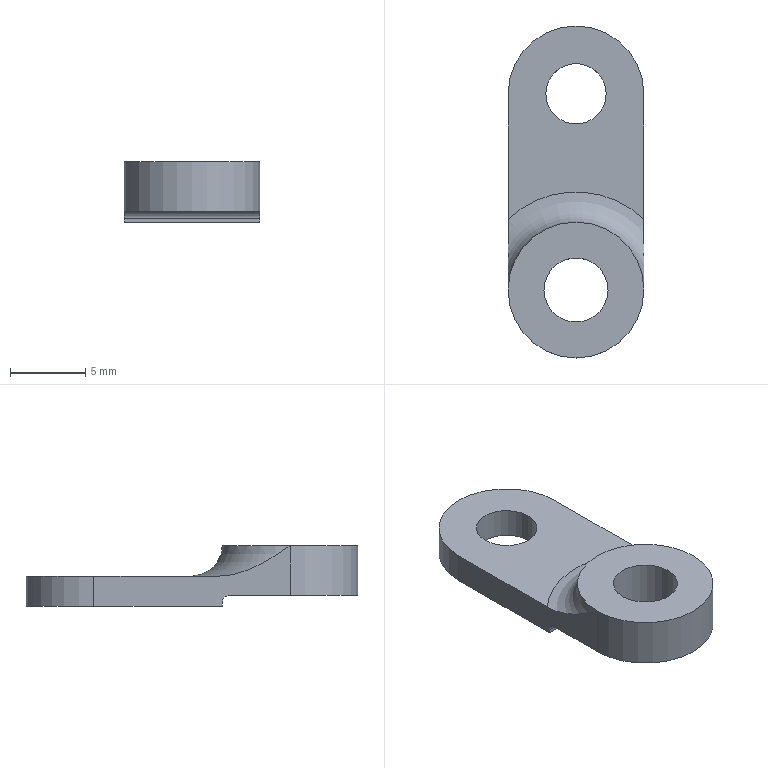NC program | NX | posted with a generic post | part box 9 x 22 x 4 mm
Whole program:
N10 G17 G21 G94 G90
(ADAPTIVE_MILLING_1 , TOOL : D10-30-D10-75-3T-FINISH)
N12 T01 M6
N14 G54
N16 G17 G0 G90 X3.609 Y-21.526 S4500 M3
N18 G43 Z1.15 H1
N20 G94 G1 X3.616 Y-21.377 Z0.213 F1500.
N22 X3.623 Y-21.227 Z-0.158
N24 X3.63 Y-21.077 Z-0.43
N26 X3.637 Y-20.927 Z-0.65
N28 X3.645 Y-20.777 Z-0.834
N30 X3.652 Y-20.627 Z-0.992
N32 X3.659 Y-20.478 Z-1.13
N34 X3.666 Y-20.328 Z-1.25
N36 X3.674 Y-20.178 Z-1.355
N38 X3.681 Y-20.028 Z-1.448
N40 X3.688 Y-19.878 Z-1.529
N42 X3.695 Y-19.728 Z-1.6
N44 X3.702 Y-19.579 Z-1.66
N46 X3.71 Y-19.429 Z-1.712
N48 X3.717 Y-19.279 Z-1.755
N50 X3.724 Y-19.129 Z-1.789
N52 X3.731 Y-18.979 Z-1.816
N54 X3.738 Y-18.83 Z-1.835
N56 X3.746 Y-18.68 Z-1.846
N58 X3.753 Y-18.53 Z-1.85
N60 X3.825 Y-17.028
N62 G3 X3.076 Y-16.003 R1.01
N64 X0.037 Y-15.742 R15.676
N66 X-13.568 Y-15.694 R849.737
N68 G2 X-17.871 Y-13.148 R5.709
N70 X-19.406 Y-8.918 R9.675
N72 X-19.687 Y-3.38 R43.207
N74 G1 X-19.688 Y9.665
N76 G2 X-17.106 Y13.908 R5.731
N78 X-12.87 Y15.415 R9.753
N80 X-7.406 Y15.687 R43.942
N82 G1 X-1.406 Y15.7
N84 X13.483 Y15.697
N86 G2 X17.786 Y13.257 R5.676
N88 X19.396 Y8.976 R9.508
N90 X19.687 Y3.363 R42.446
N92 G1 X19.688 Y-9.657
N94 G2 X17.068 Y-13.92 R5.764
N96 X12.704 Y-15.435 R9.931
N98 X6.975 Y-15.69 R48.838
N100 X1.55 Y-15.516 R62.965
N102 G3 X-7.344 Y-15.401 R225.311
N104 G2 X-12.292 Y-15.371 R114.167
N106 X-17.685 Y-11.8 R6.997
N108 X-19.122 Y-7.137 R12.027
N110 X-19.389 Y-0.921 R56.646
N112 G1 X-19.384 Y8.116
N114 G2 X-15.838 Y13.667 R6.965
N116 X-11.143 Y15.123 R11.979
N118 X-4.964 Y15.389 R56.383
N120 G1 X0.398 Y15.399
N122 G2 X12.166 Y15.38 R746.145
N124 X17.651 Y11.854 R6.984
N126 X19.118 Y7.163 R11.937
N128 X19.39 Y0.872 R56.383
N130 X19.38 Y-8.166 R448.832
N132 X15.843 Y-13.657 R6.985
N134 X11.184 Y-15.115 R11.931
N136 X2.542 Y-15.26 R51.547
N138 G3 X-10.343 Y-15.099 R304.983
N140 G2 X-17.445 Y-10.754 R7.845
N142 X-18.825 Y-5.837 R13.76
N144 X-19.089 Y0.755 R65.04
N146 X-19.07 Y7.017 R168.466
N148 X-14.85 Y13.396 R7.799
N150 X-9.944 Y14.813 R13.522
N152 X-3.766 Y15.086 R59.319
N154 G1 X1.184 Y15.099
N156 G2 X10.892 Y15.077 R558.443
N158 X17.433 Y10.77 R7.825
N160 X18.835 Y5.741 R13.864
N162 X19.089 Y-0.776 R66.532
N164 X19.07 Y-7.001 R166.156
N166 X14.828 Y-13.403 R7.812
N168 X9.805 Y-14.828 R13.709
N170 X3.25 Y-14.975 R44.243
N172 G3 X-9.446 Y-14.791 R366.794
N174 G2 X-17.181 Y-9.859 R8.509
N176 X-18.526 Y-4.733 R15.228
N178 X-18.791 Y2.459 R74.868
N180 X-18.73 Y6.357 R43.18
N182 X-13.925 Y13.15 R8.444
N184 X-8.659 Y14.535 R15.239
N186 X-1.166 Y14.792 R79.941
N188 X9.766 Y14.776 R610.284
N190 X17.168 Y9.88 R8.478
N192 X18.527 Y4.721 R15.214
N194 X18.791 Y-2.546 R75.709
N196 X18.735 Y-6.294 R44.285
N198 X13.934 Y-13.141 R8.447
N200 X8.629 Y-14.533 R15.121
N202 X2.297 Y-14.634 R51.252
N204 G3 X-8.591 Y-14.486 R621.68
N206 G2 X-14.357 Y-12.437 R9.223
N208 X-17.556 Y-7.328 R10.375
N210 X-18.376 Y-1.776 R23.819
N212 X-18.446 Y5.159 R79.772
N214 X-13.175 Y12.851 R8.97
N216 X-7.747 Y14.228 R16.352
N218 X-0.255 Y14.491 R81.917
N220 X8.904 Y14.467 R318.621
N222 X16.881 Y9.104 R9.014
N224 X18.239 Y3.634 R16.616
N226 X18.441 Y-5.208 R73.933
N228 X13.26 Y-12.806 R8.955
N230 X7.579 Y-14.222 R15.864
N232 X1.357 Y-14.304 R62.276
N234 G1 X-7.7 Y-14.185
N236 G2 X-13.037 Y-12.649 R10.181
N238 X-16.989 Y-7.401 R10.172
N240 X-18.016 Y-1.811 R21.157
N242 X-18.124 Y4.409 R54.641
N244 X-12.505 Y12.539 R9.397
N246 X-6.961 Y13.917 R17.224
N248 X0.493 Y14.188 R82.102
N250 X7.955 Y14.167 R255.277
N252 X13.789 Y12.098 R9.741
N254 X17.187 Y6.797 R10.701
N256 X18.058 Y1.139 R24.061
N258 X18.114 Y-4.52 R50.155
N260 X12.518 Y-12.529 R9.389
N262 X6.854 Y-13.884 R16.496
N264 X0.632 Y-13.984 R67.965
N266 X-7.298 Y-13.866 R417.053
N268 X-12.956 Y-11.994 R10.359
N270 X-16.735 Y-6.581 R10.758
N272 X-17.724 Y-0.831 R22.945
N274 X-17.747 Y4.225 R31.546
N276 X-12.089 Y12.127 R9.683
N278 X-6.599 Y13.567 R17.197
N280 X0.853 Y13.884 R73.619
N282 X7.452 Y13.845 R128.638
N284 X13.465 Y11.589 R10.083
N286 X16.863 Y6.169 R11.132
N288 X17.76 Y0.212 R25.388
N290 X17.721 Y-4.432 R27.272
N292 X11.998 Y-12.163 R9.675
N294 X6.19 Y-13.546 R16.957
N296 X-0.144 Y-13.666 R72.401
N298 X-6.705 Y-13.556 R181.339
N300 X-12.401 Y-11.689 R10.836
N302 X-16.338 Y-6.213 R10.97
N304 X-17.413 Y-0.176 R23.083
N306 X-17.262 Y4.571 R19.011
N308 X-11.718 Y11.708 R9.908
N310 X-6.024 Y13.245 R17.408
N312 X1.352 Y13.58 R71.272
N314 X7.05 Y13.514 R75.615
N316 X13.379 Y10.889 R10.304
N318 X16.613 Y5.329 R11.781
N320 X17.415 Y-3.484 R27.912
N322 X11.398 Y-11.847 R9.957
N324 X5.585 Y-13.209 R17.564
N326 X-0.936 Y-13.352 R75.645
N328 X-6.329 Y-13.232 R83.502
N330 X-12.306 Y-11.063 R10.975
N332 X-16.079 Y-5.474 R11.471
N334 X-17.032 Y3.159 R22.882
N336 X-11.108 Y11.417 R10.166
N338 X-5.332 Y12.941 R18.118
N340 X2.119 Y13.279 R73.326
N342 X6.989 Y13.144 R40.014
N344 X15.529 Y6.877 R10.403
N346 X16.972 Y1.037 R18.895
N348 X16.892 Y-4.082 R17.762
N350 X11.009 Y-11.443 R10.102
N352 X5.13 Y-12.865 R17.729
N354 X-2.627 Y-13.035 R85.322
N356 X-7.334 Y-12.708 R25.883
N358 X-15.176 Y-6.439 R10.653
N360 X-16.617 Y2.954 R18.961
N362 X-10.779 Y10.999 R10.29
N364 X-4.831 Y12.618 R18.184
N366 X5.693 Y12.9 R71.264
N368 X11.675 Y10.838 R11.344
N370 X15.637 Y5.284 R11.505
N372 X16.633 Y-2.807 R19.358
N374 X10.702 Y-11.008 R10.22
N376 X4.842 Y-12.508 R17.579
N378 X-5.235 Y-12.613 R70.379
N380 X-11.249 Y-10.496 R11.72
N382 X-15.352 Y-4.682 R11.811
N384 X-16.208 Y2.559 R16.692
N386 X-10.572 Y10.522 R10.343
N388 X-4.661 Y12.255 R17.668
N390 X5.184 Y12.579 R57.922
N392 X11.27 Y10.465 R11.606
N394 X15.351 Y4.67 R11.789
N396 X16.194 Y-2.645 R16.581
N398 X10.306 Y-10.62 R10.288
N400 X4.42 Y-12.166 R17.689
N402 X-4.681 Y-12.303 R57.154
N404 X-10.743 Y-10.209 R12.052
N406 X-14.998 Y-4.28 R11.945
N408 X-15.715 Y2.627 R14.386
N410 X-10.273 Y10.094 R10.362
N412 X-4.272 Y11.922 R17.545
N414 X4.821 Y12.243 R47.152
N416 X11.159 Y9.877 R11.662
N418 X14.712 Y5.046 R11.986
N420 X15.473 Y3.549 R13.977
N422 G1 X15.914 Y2.119
N424 X16.129 Y0.637
N426 G2 X14.991 Y-5.192 R13.078
N428 X9.203 Y-10.564 R10.913
N430 X3.076 Y-11.919 R20.103
N432 X-4.527 Y-11.951 R44.217
N434 X-10.975 Y-9.366 R11.848
N436 X-14.948 Y-2.866 R12.535
N438 X-14.877 Y3.864 R11.824
N440 X-9.536 Y9.902 R10.556
N442 X-3.587 Y11.631 R18.295
N444 X4.494 Y11.898 R38.875
N446 X11.015 Y9.308 R11.683
N448 X13.046 Y7.074 R11.835
N450 G1 X13.959 Y6.122
N452 X14.816 Y4.895
N454 X15.473 Y3.549
N456 X15.914 Y2.119
N458 X16.129 Y0.637
N460 X16.112 Y-0.86
N462 X15.863 Y-2.336
N464 X15.389 Y-3.757
N466 G2 X12.911 Y-7.448 R13.968
N468 X6.674 Y-10.926 R13.162
N470 X0.1 Y-11.738 R29.977
N472 X-5.428 Y-11.416 R24.678
N474 X-14. Y-4.23 R11.461
N476 X-14.533 Y3.119 R11.506
N478 X-9.349 Y9.421 R10.423
N480 X-3.363 Y11.277 R17.751
N482 X4.228 Y11.541 R32.406
N484 X11.338 Y8.327 R11.784
N486 G1 X11.731 Y8.109
N488 G2 X13.052 Y7.067 R12.874
N490 G1 X13.959 Y6.122
N492 X14.816 Y4.895
N494 X15.473 Y3.549
N496 X15.914 Y2.119
N498 X16.129 Y0.637
N500 X16.112 Y-0.86
N502 X15.863 Y-2.336
N504 X15.389 Y-3.757
N506 X14.701 Y-5.086
N508 X13.815 Y-6.293
N510 G2 X12.548 Y-7.512 R16.368
N512 X4.238 Y-11.016 R17.399
N514 X-3.911 Y-11.26 R31.391
N516 X-11.036 Y-7.884 R11.805
N518 X-14.332 Y1.255 R11.547
N520 X-9.499 Y8.725 R10.08
N522 X-3.562 Y10.851 R16.39
N524 X3.945 Y11.179 R27.757
N526 X9.599 Y9.119 R12.485
N528 X11.375 Y8.304 R8.087
N530 G1 X11.731 Y8.109
N532 X12.923 Y7.202
N534 X13.959 Y6.122
N536 X14.816 Y4.895
N538 X15.473 Y3.549
N540 X15.914 Y2.119
N542 X16.129 Y0.637
N544 X16.112 Y-0.86
N546 X15.863 Y-2.336
N548 X15.389 Y-3.757
N550 X14.701 Y-5.086
N552 X13.815 Y-6.293
N554 X12.754 Y-7.349
N556 X11.542 Y-8.228
N558 G2 X9.056 Y-9.337 R13.408
N560 X-0.377 Y-11.061 R27.845
N562 X-6.152 Y-10.327 R17.05
N564 X-13.84 Y0.109 R11.087
N566 X-9.54 Y8.049 R9.78
N568 X-3.705 Y10.415 R15.309
N570 X3.978 Y10.767 R23.589
N572 X8.028 Y9.518 R14.933
N574 G1 X9.227 Y9.257
N576 X9.649 Y9.099
N578 G3 X10.391 Y9.115 R1.004
N580 G1 X11.182 Y9.452
N582 X13.013 Y10.232 Z-1.75
N584 G2 X13.839 Y10.312 R1.09 F15000.
N586 G1 X13.972 Y10.257
N588 X14.665 Y9.914
N590 X15.35 Y9.556
N592 G2 X16.83 Y8.076 R4.232
N594 G1 X17.426 Y7.074
N596 X18.01 Y6.066
N598 G2 X19.247 Y0.691 R10.545
N600 X18.986 Y-2.108 R18.384
N602 X17.766 Y-5.979 R16.637
N604 X15.976 Y-8.565 R9.892
N606 G1 X14.549 Y-10.05
N608 G2 X13.343 Y-10.232 R1.
N610 G1 X13.173 Y-10.138
N612 X11.433 Y-9.173 Z-1.85 F1500.
N614 X11.179 Y-9.03
N616 X10.919 Y-8.899
N618 G3 X10.226 Y-8.892 R1.005
N620 G2 X7.944 Y-9.533 R10.005
N622 X-0.519 Y-10.708 R37.607
N624 X-6.473 Y-9.716 R15.368
N626 X-13.163 Y-1.445 R10.74
N628 X-9.594 Y7.309 R9.43
N630 X-3.728 Y9.986 R14.343
N632 X3.906 Y10.353 R20.559
N634 X6.695 Y9.637 R22.554
N636 X8.061 Y9.511 R11.524
N638 G3 X9.011 Y9.812 R1.001
N640 G1 X9.154 Y9.967
N642 X10.499 Y11.433 Z-1.75
N644 G2 X10.865 Y11.772 R1.702 F15000.
N646 X11.938 Y11.749 R1.001
N648 G1 X12.935 Y11.087
N650 X13.923 Y10.412
N652 G2 X16.214 Y8.229 R12.234
N654 G1 X16.735 Y7.588
N656 X17.244 Y6.937
N658 G2 X18.55 Y3.99 R7.734
N660 X19.13 Y-0.795 R29.213
N662 X18.278 Y-5.056 R9.998
N664 X16.899 Y-7.52 R11.692
N666 X14.525 Y-9.845 R10.7
N668 G1 X11.821 Y-11.771
N670 G2 X10.497 Y-11.626 R1.
N672 G1 X10.381 Y-11.497
N674 X9.05 Y-10.018 Z-1.85 F1500.
N676 G3 X8.663 Y-9.654 R1.728
N678 X7.944 Y-9.533 R1.004
N680 X3.672 Y-10.066 R78.278
N682 G2 X-2.648 Y-10.225 R26.549
N684 X-9.664 Y-7.04 R11.853
N686 X-12.598 Y0.743 R9.484
N688 X-8.575 Y7.371 R9.483
N690 X-2.489 Y9.818 R15.057
N692 X5.231 Y9.653 R17.976
N694 G1 X6.762 Y9.631
N696 G3 X7.688 Y10.109 R1.001
N698 G1 X7.795 Y10.343 Z-1.837
N700 X7.876 Y10.587 Z-1.824
N702 X8.349 Y11.983 Z-1.75
N704 X8.422 Y12.198 F15000.
N706 X8.506 Y12.41
N708 G2 X9.927 Y12.796 R1.
N710 G1 X13.083 Y10.807
N712 G2 X15.397 Y9.073 R17.516
N714 X16.735 Y7.515 R8.834
N716 G1 X17.197 Y6.829
N718 X17.652 Y6.137
N720 G2 X18.811 Y3.327 R10.14
N722 X19.158 Y1.249 R15.517
N724 X18.984 Y-2.424 R10.937
N726 G1 X18.816 Y-3.188
N728 X18.636 Y-3.951
N730 G2 X16.028 Y-8.457 R10.101
N732 G1 X15.267 Y-9.221
N734 X14.497 Y-9.976
N736 G2 X12.354 Y-11.306 R7.1
N738 G1 X10.987 Y-11.846
N740 G2 X9.943 Y-11.653 R1.003
N742 G1 X8.431 Y-10.36 Z-1.85 F1500.
N744 X8.082 Y-10.059
N746 X7.726 Y-9.768
N748 G3 X7.111 Y-9.608 R1.008
N750 G2 X5.127 Y-9.68 R68.884
N752 X-0.003 Y-9.998 R71.011
N754 X-6.006 Y-8.885 R14.746
N756 X-11.52 Y-3.148 R9.986
N758 X-9.288 Y5.994 R8.737
N760 X-3.526 Y9.141 R12.805
N762 X2.958 Y9.65 R18.4
N764 G1 X5.283
N766 G3 X6.177 Y10.201 R1.001
N768 G1 X6.235 Y10.317
N770 X7.128 Y12.095 Z-1.75
N772 G2 X7.401 Y12.549 R1.819 F15000.
N774 X8.449 Y12.815 R1.001
N776 G1 X10.096 Y12.257
N778 G2 X11.896 Y11.428 R13.802
N780 G1 X12.916 Y10.868
N782 X13.928 Y10.295
N784 G2 X17.864 Y5.881 R10.408
N786 G1 X18.051 Y5.459
N788 X18.223 Y5.031
N790 X18.628 Y3.951
N792 X19.019 Y2.866
N794 G2 X19.331 Y-1.499 R9.297
N796 X17.745 Y-6.143 R15.121
N798 X16.972 Y-7.484 R14.242
N800 X15.112 Y-9.476 R8.835
N802 X11.979 Y-11.401 R16.21
N804 G1 X8.952 Y-12.815
N806 G2 X7.614 Y-12.313 R1.
N808 G1 X7.518 Y-12.096
N810 X6.715 Y-10.276 Z-1.85 F1500.
N812 G3 X5.787 Y-9.65 R1.002
N814 G2 X-0.169 Y-9.661 R585.998
N816 X-6.117 Y-8.3 R14.161
N818 X-10.918 Y-2.944 R9.33
N820 X-8.87 Y5.519 R8.439
N822 X-3.157 Y8.767 R12.215
N824 X0.956 Y9.34 R18.49
N826 G1 X1.769 Y9.553
N828 X2.928 Y9.648
N830 G3 X3.739 Y11.095 R1.
N832 X3.144 Y11.604 Z-1.81 R1.062
N834 G1 X2.051 Y12.065 Z-1.75
N836 X0.394 Y12.764 F15000.
N838 G3 X-0.237 Y12.813 R1.008
N840 G1 X-1.503 Y12.497
N842 X-2.766 Y12.169
N844 G3 X-6.71 Y10.687 R24.054
N846 X-9.302 Y9.165 R19.306
N848 X-11.633 Y7.021 R12.861
N850 X-12.537 Y5.895 R13.742
N852 X-14.051 Y2.1 R9.362
N854 G1 X-14.457 Y-0.354
N856 G3 X-14.228 Y-3.179 R6.023
N858 X-13.403 Y-5.062 R9.368
N860 G1 X-12.732 Y-6.228
N862 X-12.049 Y-7.387
N864 G3 X-9.826 Y-9.794 R9.055
N866 X-8.781 Y-10.446 R8.525
N868 X-6.289 Y-11.587 R18.612
N870 X-4.768 Y-12.051 R16.768
N872 X-2.741 Y-12.512 R25.947
N874 G1 X-2.111 Y-12.608
N876 X-1.478 Y-12.686
N878 X-0.783 Y-12.76
N880 X-0.087 Y-12.82
N882 X0.089 Y-12.8
N884 X0.26 Y-12.751
N886 X1.968 Y-12.081
N888 X2.645 Y-11.819 Z-1.787 F1500.
N890 X3.319 Y-11.545 Z-1.823
N892 G3 X3.718 Y-11.199 Z-1.85 R1.005
N894 X2.959 Y-9.65 R1.
N896 G2 X-1.901 Y-9.168 R75.766
N898 X-7.534 Y-6.777 R11.739
N900 X-8.689 Y4.717 R8.038
N902 X-2.999 Y8.312 R11.292
N904 X-0.24 Y8.868 R24.521
N906 G1 X0.614 Y9.251
N908 X0.977 Y9.346
N910 G3 X1.369 Y11.077 R1.
N912 X0.723 Y11.318 Z-1.815 R1.083
N914 G1 X-0.558 Y11.443 Z-1.75
N916 X-2.486 Y11.63 F15000.
N918 G3 X-2.899 Y11.584 R1.055
N920 G1 X-4.078 Y11.193
N922 X-5.253 Y10.788
N924 G3 X-8.435 Y9.21 R17.097
N926 X-10.837 Y7.067 R10.728
N928 G1 X-11.382 Y6.412
N930 X-11.915 Y5.748
N932 G3 X-13.768 Y1.093 R9.744
N934 X-12.956 Y-4.312 R10.16
N936 G1 X-12.673 Y-4.942
N938 X-12.381 Y-5.568
N940 G3 X-10.116 Y-8.539 R10.238
N942 X-7.333 Y-10.496 R13.057
N944 X-3.472 Y-12.094 R19.805
N946 G1 X-1.305 Y-12.733
N948 G3 X-0.611 Y-12.685 R1.005
N950 G1 X1.007 Y-11.954
N952 X2.151 Y-11.432 Z-1.813 F1500.
N954 G3 X2.621 Y-10.893 Z-1.85 R1.001
N956 X1.86 Y-9.568 R1.
N958 G2 X-2.68 Y-8.653 R81.122
N960 X-7.616 Y-5.936 R10.633
N962 X-8.295 Y4.06 R7.686
N964 X-2.894 Y7.812 R10.473
N966 G3 X-1.03 Y8.373 R30.332
N968 G2 X-0.13 Y8.909 R4.424
N970 G3 X0.29 Y10.366 R1.
N972 X-0.479 Y10.821 Z-1.804 R1.046
N974 G1 X-1.531 Y10.994 Z-1.75
N976 X-3.31 Y11.288 F15000.
N978 G3 X-4.006 Y11.147 R1.005
N980 G1 X-7.161 Y9.158
N982 G3 X-9.476 Y7.424 R17.516
N984 X-10.814 Y5.866 R8.834
N986 X-11.64 Y4.563 R15.292
N988 X-12.622 Y1.986 R10.125
N990 G1 X-12.81 Y1.182
N992 X-12.983 Y0.376
N994 G3 X-12.768 Y-3.302 R8.061
N996 X-11.431 Y-6.232 R10.863
N998 X-10.609 Y-7.418 R13.301
N1000 X-9.057 Y-8.883 R8.532
N1002 X-7.38 Y-9.936 R12.501
N1004 G1 X-2.39 Y-12.536
N1006 G3 X-1.442 Y-12.523 R1.001
N1008 G1 X-0.035 Y-11.741
N1010 X1.008 Y-11.155 Z-1.81 F1500.
N1012 G3 X1.442 Y-10.517 Z-1.85 R1.
N1014 X0.775 Y-9.37 R1.
N1016 X-2.644 Y-8.324 R155.82
N1018 G2 X-6.96 Y-5.762 R10.374
N1020 X-7.609 Y3.723 R7.414
N1022 X-3.146 Y7.165 R10.112
N1024 G3 X-1.719 Y7.804 R11.055
N1026 G1 X-1.633 Y7.876
N1028 G3 X-1.447 Y9.058 R1.
N1030 X-2.199 Y9.587 Z-1.802 R1.043
N1032 G1 X-3.209 Y9.819 Z-1.75
N1034 X-4.838 Y10.194 F15000.
N1036 G3 X-5.509 Y10.114 R1.006
N1038 G1 X-6.281 Y9.718
N1040 G3 X-7.042 Y9.101 R3.435
N1042 G1 X-8.065 Y7.992
N1044 X-9.076 Y6.873
N1046 G3 X-11.294 Y3.285 R13.688
N1048 X-12.135 Y-0.165 R11.525
N1050 X-11.579 Y-4.239 R9.662
N1052 X-10.503 Y-6.261 R8.86
N1054 G1 X-9.787 Y-7.273
N1056 X-9.056 Y-8.274
N1058 G3 X-5.906 Y-10.576 R7.395
N1060 G1 X-3.816 Y-11.373
N1062 G3 X-3.323 Y-11.429 R1.02
N1064 G1 X-1.439 Y-11.168
N1066 X-0.207 Y-10.994 Z-1.813 F1500.
N1068 G3 X0.403 Y-10.598 Z-1.85 R1.001
N1070 X0.06 Y-9.134 R1.
N1072 X-2.354 Y-8.123 R20.94
N1074 G2 X-6.201 Y-5.697 R10.501
N1076 X-6.753 Y3.556 R7.189
N1078 X-3.31 Y6.511 R10.677
N1080 G3 X-2.217 Y7.214 R7.881
N1082 G1 X-1.454 Y8.074
N1084 X-0.96 Y8.415
N1086 G3 X-0.967 Y10.065 R1.
N1088 X-1.747 Y10.218 Z-1.809 R1.061
N1090 G1 X-2.913 Y10.076 Z-1.75
N1092 X-4.698 Y9.859 F15000.
N1094 G3 X-5.284 Y9.573 R1.007
N1096 G1 X-6.582 Y8.28
N1098 X-7.868 Y6.974
N1100 G3 X-10.787 Y2.273 R14.546
N1102 G1 X-11.452 Y0.53
N1104 G3 X-11.619 Y-1.844 R4.111
N1106 X-10.747 Y-4.148 R8.961
N1108 G1 X-9.163 Y-7.047
N1110 G3 X-6.096 Y-10.123 R7.755
N1112 G1 X-4.114 Y-11.214
N1114 G3 X-3.47 Y-11.324 R1.007
N1116 G1 X-1.697 Y-11.033
N1118 X-0.48 Y-10.829 Z-1.812 F1500.
N1120 G3 X0.126 Y-10.41 Z-1.85 R1.001
N1122 X-0.238 Y-8.976 R1.
N1124 X-3.147 Y-7.431 R91.588
N1126 G2 X-6.639 Y-3.914 R8.156
N1128 X-5.906 Y3.336 R7.122
N1130 X-3.163 Y6.052 R13.582
N1132 G3 X-2.466 Y6.933 R3.227
N1134 G1 X-2.192 Y7.241
N1136 G3 X-2.698 Y8.875 R1.
N1138 X-3.439 Y8.776 Z-1.812 R1.062
N1140 G1 X-4.555 Y8.27 Z-1.75
N1142 X-6.374 Y7.445 F15000.
N1144 X-6.53 Y7.355
N1146 X-6.668 Y7.241
N1148 X-7.254 Y6.657
N1150 X-7.832 Y6.064
N1152 G3 X-9.932 Y2.106 R8.875
N1154 X-10.242 Y0.595 R15.077
N1156 X-10.239 Y-2.162 R9.991
N1158 G1 X-10.124 Y-3.005
N1160 X-9.991 Y-3.844
N1162 G3 X-8.586 Y-6.788 R6.693
N1164 X-6.254 Y-9.001 R11.226
N1166 G1 X-4.928 Y-9.939
N1168 G3 X-4.492 Y-10.112 R1.026
N1170 G1 X-2.615 Y-10.38
N1172 X-1.288 Y-10.564 Z-1.817 F1500.
N1174 G3 X-0.67 Y-10.406 Z-1.85 R1.002
N1176 X-0.604 Y-8.78 R1.
N1178 X-2.779 Y-7.311 R23.541
N1180 G2 X-5.927 Y-3.714 R8.03
N1182 X-5.327 Y2.765 R7.227
N1184 X-3.662 Y4.973 R16.567
N1186 X-2.856 Y6.35 R6.867
N1188 G3 X-3.21 Y7.786 R1.
N1190 X-4.119 Y7.814 Z-1.803 R1.044
N1192 G1 X-5.102 Y7.455 Z-1.75
N1194 X-6.781 Y6.843 F15000.
N1196 G3 X-7.333 Y6.35 R1.004
N1198 G1 X-7.722 Y5.573
N1200 X-8.101 Y4.791
N1202 G3 X-8.76 Y2.924 R12.121
N1204 X-9.553 Y-1.963 R21.286
N1206 X-9.009 Y-4.736 R5.686
N1208 X-7.923 Y-6.476 R8.111
N1210 G1 X-5.372 Y-9.593
N1212 G3 X-4.687 Y-9.956 R1.003
N1214 G1 X-2.924 Y-10.115
N1216 X-1.684 Y-10.221 Z-1.813 F1500.
N1218 G3 X-1.001 Y-9.974 Z-1.85 R1.001
N1220 X-1.048 Y-8.435 R1.
N1222 X-3.106 Y-6.685 R178.362
N1224 G2 X-5.015 Y1.67 R7.313
N1226 G1 X-4.462 Y2.872
N1228 X-3.988 Y4.295
N1230 X-3.608 Y5.069
N1232 G3 X-4.499 Y6.51 R1.
N1234 X-5.193 Y6.243 Z-1.812 R1.063
N1236 G1 X-6.165 Y5.491 Z-1.75
N1238 X-7.595 Y4.386 F15000.
N1240 G3 X-7.932 Y3.911 R1.01
N1242 G1 X-8.195 Y3.127
N1244 X-8.445 Y2.338
N1246 G3 X-8.739 Y0.309 R8.134
N1248 X-8.674 Y-1.897 R15.776
N1250 X-7.73 Y-5.468 R13.442
N1252 X-6.789 Y-7.366 R15.352
N1254 G1 X-5.599 Y-9.395
N1256 G3 X-4.749 Y-9.889 R1.001
N1258 G1 X-3.139 Y-9.909
N1260 X-1.943 Y-9.918 Z-1.81 F1500.
N1262 G3 X-1.249 Y-9.581 Z-1.85 R1.
N1264 X-1.275 Y-8.236 R1.
N1266 G2 X-3.446 Y-5.769 R23.333
N1268 X-4.805 Y-0.508 R7.755
N1270 G1 X-4.832 Y-0.177
N1272 X-4.753 Y1.347
N1274 X-4.458 Y2.883
N1276 G3 X-5.689 Y4.158 R1.
N1278 X-6.263 Y3.724 Z-1.813 R1.067
N1280 G1 X-7.019 Y2.723 Z-1.75
N1282 X-8.133 Y1.247 F15000.
N1284 G3 X-8.335 Y0.645 R1.008
N1286 G1 X-8.325 Y-0.286
N1288 G3 X-8.187 Y-1.203 R5.493
N1290 G1 X-6.722 Y-7.209
N1292 G3 X-6.042 Y-7.928 R1.001
N1294 G1 X-4.459 Y-8.41
N1296 X-3.282 Y-8.763 Z-1.812 F1500.
N1298 G3 X-2.549 Y-8.652 Z-1.85 R1.001
N1300 X-2.246 Y-7.209 R1.
N1302 G1 X-3.135 Y-5.968
N1304 X-3.849 Y-4.62
N1306 X-4.376 Y-3.187
N1308 X-4.706 Y-1.697
N1310 X-4.805 Y-0.502
N1312 G3 X-5.598 Y0.402 R1.01
N1314 G1 X-7.273 Y0.764
N1316 X-7.42 Y0.796 Z-1.846
N1318 X-7.567 Y0.828 Z-1.835
N1320 X-7.713 Y0.859 Z-1.816
N1322 X-7.86 Y0.891 Z-1.789
N1324 X-8.007 Y0.923 Z-1.755
N1326 X-8.153 Y0.954 Z-1.712
N1328 X-8.3 Y0.986 Z-1.66
N1330 X-8.446 Y1.018 Z-1.6
N1332 X-8.593 Y1.049 Z-1.529
N1334 X-8.74 Y1.081 Z-1.448
N1336 X-8.886 Y1.113 Z-1.355
N1338 X-9.033 Y1.144 Z-1.25
N1340 X-9.179 Y1.176 Z-1.13
N1342 X-9.326 Y1.208 Z-0.992
N1344 X-9.473 Y1.24 Z-0.834
N1346 X-9.619 Y1.271 Z-0.65
N1348 X-9.766 Y1.303 Z-0.43
N1350 X-9.912 Y1.335 Z-0.158
N1352 X-10.059 Y1.366 Z0.213
N1354 X-10.206 Y1.398 Z1.15
N1356 G0 X4.304 Y-15.127 Z1.638
N1358 G1 X4.316 Y-14.977 Z0.701
N1360 X4.328 Y-14.828 Z0.33
N1362 X4.34 Y-14.678 Z0.057
N1364 X4.352 Y-14.529 Z-0.163
N1366 X4.364 Y-14.379 Z-0.347
N1368 X4.376 Y-14.23 Z-0.505
N1370 X4.389 Y-14.08 Z-0.642
N1372 X4.401 Y-13.931 Z-0.763
N1374 X4.413 Y-13.781 Z-0.868
N1376 X4.425 Y-13.632 Z-0.961
N1378 X4.437 Y-13.482 Z-1.042
N1380 X4.449 Y-13.333 Z-1.112
N1382 X4.461 Y-13.183 Z-1.173
N1384 X4.474 Y-13.034 Z-1.224
N1386 X4.486 Y-12.884 Z-1.267
N1388 X4.498 Y-12.735 Z-1.302
N1390 X4.51 Y-12.585 Z-1.329
N1392 X4.522 Y-12.436 Z-1.347
N1394 X4.534 Y-12.286 Z-1.359
N1396 X4.546 Y-12.137 Z-1.363
N1398 X4.664 Y-10.694
N1400 G3 X3.734 Y-9.605 R1.01
N1402 G2 X-1.427 Y-7.094 R8.054
N1404 X-3.404 Y4.253 R10.405
N1406 X0.386 Y8.219 R7.19
N1408 G1 X1.533 Y8.964
N1410 G2 X3.34 Y9.575 R6.745
N1412 G1 X3.751 Y9.607
N1414 G3 X4.031 Y11.538 R1.
N1416 G1 X3.773 Y11.6 Z-1.349
N1418 X3.509 Y11.633 Z-1.336
N1420 X2.063 Y11.815 Z-1.263
N1422 X0.555 Y12.005 F15000.
N1424 G3 X-0.125 Y11.845 R1.005
N1426 G1 X-1.122 Y11.183
N1428 X-2.11 Y10.508
N1430 G3 X-6.985 Y2.606 R12.355
N1432 G1 X-7.057 Y2.083
N1434 X-7.11 Y1.557
N1436 X-7.185 Y0.571
N1438 X-7.245 Y-0.417
N1440 G3 X-5.277 Y-7.216 R11.679
N1442 X-2.874 Y-9.881 R12.183
N1444 G1 X-0.525 Y-11.814
N1446 G3 X0.273 Y-12.029 R1.002
N1448 G1 X1.831 Y-11.772
N1450 X3.338 Y-11.519 Z-1.339 F1500.
N1452 G3 X3.748 Y-11.318 Z-1.363 R1.014
N1454 X3.351 Y-9.576 R1.
N1456 G2 X1.526 Y-8.96 R6.767
N1458 X0.156 Y-8.044 R35.485
N1460 X-1.855 Y-5.932 R11.446
N1462 X-2.974 Y3.888 R10.26
N1464 G1 X-2.474 Y4.949
N1466 G2 X-0.754 Y7.239 R11.943
N1468 G1 X0.392 Y8.223
N1470 G3 X-0.421 Y10.025 R1.
N1472 G1 X-0.847 Y9.852 Z-1.339
N1474 X-1.267 Y9.664 Z-1.316
N1476 X-2.245 Y9.233 Z-1.263
N1478 X-3.63 Y8.623 F15000.
N1480 G3 X-4.085 Y8.223 R1.009
N1482 G1 X-4.224 Y7.994
N1484 X-4.335 Y7.75
N1486 X-4.363 Y7.632
N1488 X-4.617 Y6.211
N1490 X-4.968 Y4.252 Z-1.363 F1500.
N1492 G3 X-3.078 Y3.647 R1.
N1494 G1 X-2.841 Y4.157
N1496 G3 X-4.878 Y4.98 R-1.1
N1498 G1 X-5.592 Y2.925
N1500 G3 X-3.499 Y2.247 R-1.1
N1502 G1 X-3.153 Y3.396
N1504 G3 X-5.281 Y3.947 R-1.1
N1506 G1 X-5.88 Y1.199
N1508 G3 X-3.717 Y0.801 R-1.1
N1510 G1 X-3.51 Y2.173
N1512 G3 X-5.695 Y2.421 R-1.1
N1514 G1 X-5.924 Y-0.569
N1516 G3 X-3.727 Y-0.661 R-1.1
N1518 G1 X-3.718 Y0.689
N1520 G3 X-5.915 Y0.623 R-1.1
N1522 G1 X-5.716 Y-2.332
N1524 G3 X-3.529 Y-2.11 R-1.1
N1526 G1 X-3.712 Y-0.772
N1528 G3 X-5.878 Y-1.15 R-1.1
N1530 G1 X-5.26 Y-4.047
N1532 G3 X-3.127 Y-3.515 R-1.1
N1534 G1 X-3.488 Y-2.253
N1536 G3 X-5.577 Y-2.937 R-1.1
N1538 G1 X-4.564 Y-5.68
N1540 G3 X-2.529 Y-4.849 R-1.1
N1542 G1 X-3.066 Y-3.652
N1544 G3 X-5.036 Y-4.626 R-1.1
N1546 G1 X-3.643 Y-7.197
N1548 G3 X-1.747 Y-6.085 R-1.1
N1550 G1 X-2.408 Y-5.039
N1552 G3 X-4.219 Y-6.286 R-1.1
N1554 G1 X-2.515 Y-8.569
N1556 G3 X-0.797 Y-7.196 R-1.1
N1558 G1 X-1.503 Y-6.37
N1560 G3 X-3.115 Y-7.864 R-1.1
N1562 G1 X-1.2 Y-9.768
N1564 G3 X0.302 Y-8.162 R-1.1
N1566 G1 X-0.318 Y-7.617
N1568 G3 X-1.595 Y-7.571 R1.01
N1570 G1 X-2.901 Y-8.562
N1572 X-3.021 Y-8.652 Z-1.359
N1574 X-3.14 Y-8.743 Z-1.347
N1576 X-3.26 Y-8.833 Z-1.329
N1578 X-3.379 Y-8.924 Z-1.302
N1580 X-3.499 Y-9.015 Z-1.267
N1582 X-3.618 Y-9.105 Z-1.224
N1584 X-3.738 Y-9.196 Z-1.173
N1586 X-3.857 Y-9.287 Z-1.112
N1588 X-3.977 Y-9.377 Z-1.042
N1590 X-4.096 Y-9.468 Z-0.961
N1592 X-4.216 Y-9.559 Z-0.868
N1594 X-4.335 Y-9.649 Z-0.763
N1596 X-4.455 Y-9.74 Z-0.642
N1598 X-4.574 Y-9.831 Z-0.505
N1600 X-4.694 Y-9.921 Z-0.347
N1602 X-4.813 Y-10.012 Z-0.163
N1604 X-4.933 Y-10.102 Z0.057
N1606 X-5.052 Y-10.193 Z0.33
N1608 X-5.172 Y-10.284 Z0.701
N1610 X-5.292 Y-10.374 Z1.638
N1612 G0 X6.172 Y-15.129 Z2.125
N1614 G1 X6.161 Y-14.979 Z1.188
N1616 X6.151 Y-14.83 Z0.817
N1618 X6.14 Y-14.68 Z0.545
N1620 X6.129 Y-14.53 Z0.325
N1622 X6.118 Y-14.381 Z0.141
N1624 X6.107 Y-14.231 Z-0.017
N1626 X6.097 Y-14.082 Z-0.155
N1628 X6.086 Y-13.932 Z-0.275
N1630 X6.075 Y-13.782 Z-0.38
N1632 X6.064 Y-13.633 Z-0.473
N1634 X6.053 Y-13.483 Z-0.554
N1636 X6.042 Y-13.334 Z-0.625
N1638 X6.032 Y-13.184 Z-0.685
N1640 X6.021 Y-13.034 Z-0.737
N1642 X6.01 Y-12.885 Z-0.78
N1644 X5.999 Y-12.735 Z-0.814
N1646 X5.988 Y-12.586 Z-0.841
N1648 X5.978 Y-12.436 Z-0.86
N1650 X5.967 Y-12.286 Z-0.871
N1652 X5.956 Y-12.137 Z-0.875
N1654 X5.842 Y-10.565
N1656 G3 X4.927 Y-9.632 R1.01
N1658 G2 X3.425 Y-9.379 R6.247
N1660 G1 X2.06 Y-8.815
N1662 X0.794 Y-8.053
N1664 X-0.344 Y-7.112
N1666 X-1.329 Y-6.011
N1668 X-2.138 Y-4.775
N1670 X-2.754 Y-3.433
N1672 X-3.162 Y-2.013
N1674 X-3.355 Y-0.549
N1676 X-3.326 Y0.928
N1678 X-3.078 Y2.384
N1680 X-2.635 Y3.737
N1682 X-2.003 Y5.012
N1684 X-1.194 Y6.182
N1686 X-0.224 Y7.225
N1688 X0.885 Y8.117
N1690 X2.11 Y8.84
N1692 X3.428 Y9.38
N1694 G2 X4.956 Y9.632 R6.237
N1696 G3 X5.875 Y10.562 R1.01
N1698 G1 X5.994 Y12.137
N1700 X6.006 Y12.286 Z-0.871
N1702 X6.017 Y12.436 Z-0.86
N1704 X6.028 Y12.585 Z-0.841
N1706 X6.04 Y12.735 Z-0.814
N1708 X6.051 Y12.885 Z-0.78
N1710 X6.062 Y13.034 Z-0.737
N1712 X6.074 Y13.184 Z-0.685
N1714 X6.085 Y13.333 Z-0.625
N1716 X6.096 Y13.483 Z-0.554
N1718 X6.108 Y13.632 Z-0.473
N1720 X6.119 Y13.782 Z-0.38
N1722 X6.13 Y13.932 Z-0.275
N1724 X6.142 Y14.081 Z-0.155
N1726 X6.153 Y14.231 Z-0.017
N1728 X6.164 Y14.38 Z0.141
N1730 X6.176 Y14.53 Z0.325
N1732 X6.187 Y14.679 Z0.545
N1734 X6.198 Y14.829 Z0.817
N1736 X6.21 Y14.979 Z1.188
N1738 X6.221 Y15.128 Z2.125
N1740 G0 X6.986 Y-15.095 Z2.613
N1742 G1 X6.961 Y-14.947 Z1.676
N1744 X6.936 Y-14.799 Z1.305
N1746 X6.911 Y-14.651 Z1.032
N1748 X6.887 Y-14.503 Z0.813
N1750 X6.862 Y-14.355 Z0.628
N1752 X6.837 Y-14.208 Z0.47
N1754 X6.812 Y-14.06 Z0.333
N1756 X6.787 Y-13.912 Z0.213
N1758 X6.762 Y-13.764 Z0.107
N1760 X6.737 Y-13.616 Z0.014
N1762 X6.712 Y-13.468 Z-0.067
N1764 X6.687 Y-13.32 Z-0.137
N1766 X6.662 Y-13.172 Z-0.198
N1768 X6.637 Y-13.024 Z-0.249
N1770 X6.612 Y-12.876 Z-0.292
N1772 X6.587 Y-12.728 Z-0.327
N1774 X6.563 Y-12.58 Z-0.354
N1776 X6.538 Y-12.433 Z-0.372
N1778 X6.513 Y-12.285 Z-0.384
N1780 X6.488 Y-12.137 Z-0.388
N1782 X6.202 Y-10.439
N1784 G3 X5.373 Y-9.61 R1.01
N1786 G1 X4.192 Y-9.412
N1788 X2.826 Y-8.968
N1790 X1.541 Y-8.326
N1792 X0.365 Y-7.502
N1794 X-0.676 Y-6.513
N1796 X-1.56 Y-5.381
N1798 X-2.266 Y-4.131
N1800 X-2.781 Y-2.79
N1802 X-3.091 Y-1.388
N1804 X-3.191 Y0.045
N1806 X-3.078 Y1.476
N1808 X-2.757 Y2.866
N1810 X-2.236 Y4.194
N1812 X-1.526 Y5.431
N1814 X-0.642 Y6.55
N1816 X0.397 Y7.528
N1818 X1.568 Y8.342
N1820 X2.846 Y8.976
N1822 X4.203 Y9.415
N1824 X5.387 Y9.613
N1826 G3 X6.216 Y10.439 R1.01
N1828 G1 X6.506 Y12.137
N1830 X6.531 Y12.284 Z-0.384
N1832 X6.557 Y12.432 Z-0.372
N1834 X6.582 Y12.58 Z-0.354
N1836 X6.607 Y12.728 Z-0.327
N1838 X6.632 Y12.876 Z-0.292
N1840 X6.658 Y13.024 Z-0.249
N1842 X6.683 Y13.172 Z-0.198
N1844 X6.708 Y13.319 Z-0.137
N1846 X6.733 Y13.467 Z-0.067
N1848 X6.759 Y13.615 Z0.014
N1850 X6.784 Y13.763 Z0.107
N1852 X6.809 Y13.911 Z0.213
N1854 X6.834 Y14.059 Z0.333
N1856 X6.86 Y14.207 Z0.47
N1858 X6.885 Y14.354 Z0.628
N1860 X6.91 Y14.502 Z0.813
N1862 X6.936 Y14.65 Z1.032
N1864 X6.961 Y14.798 Z1.305
N1866 X6.986 Y14.946 Z1.676
N1868 X7.011 Y15.094 Z2.613
N1870 G0 X7.062 Y-15.178 Z3.1
N1872 G1 X7.069 Y-15.028 Z2.163
N1874 X7.076 Y-14.879 Z1.792
N1876 X7.083 Y-14.729 Z1.52
N1878 X7.09 Y-14.579 Z1.3
N1880 X7.097 Y-14.429 Z1.116
N1882 X7.103 Y-14.279 Z0.958
N1884 X7.11 Y-14.129 Z0.82
N1886 X7.117 Y-13.979 Z0.7
N1888 X7.124 Y-13.83 Z0.595
N1890 X7.131 Y-13.68 Z0.502
N1892 X7.137 Y-13.53 Z0.421
N1894 X7.144 Y-13.38 Z0.35
N1896 X7.151 Y-13.23 Z0.29
N1898 X7.158 Y-13.08 Z0.238
N1900 X7.165 Y-12.931 Z0.195
N1902 X7.172 Y-12.781 Z0.161
N1904 X7.178 Y-12.631 Z0.134
N1906 X7.185 Y-12.481 Z0.115
N1908 X7.192 Y-12.331 Z0.104
N1910 X7.199 Y-12.181 Z0.1
N1912 X7.268 Y-10.676
N1914 G3 X6.522 Y-9.655 R1.01
N1916 X5.082 Y-9.507 R8.164
N1918 G1 X3.671 Y-9.186
N1920 X2.325 Y-8.657
N1922 X1.072 Y-7.933
N1924 X-0.057 Y-7.028
N1926 X-1.037 Y-5.964
N1928 X-1.847 Y-4.765
N1930 X-2.468 Y-3.459
N1932 X-2.885 Y-2.073
N1934 X-3.09 Y-0.641
N1936 X-3.078 Y0.806
N1938 X-2.852 Y2.218
N1940 X-2.419 Y3.582
N1942 X-1.789 Y4.866
N1944 X-0.975 Y6.042
N1946 X0.005 Y7.085
N1948 X1.128 Y7.97
N1950 X2.371 Y8.679
N1952 X3.705 Y9.196
N1954 X5.1 Y9.509
N1956 X6.527 Y9.612
N1958 G2 X9.2 Y9.225 R11.187
N1960 X11.66 Y8.109 R11.186
N1962 G1 X12.855 Y7.211
N1964 X13.895 Y6.139
N1966 X14.757 Y4.919
N1968 X15.42 Y3.58
N1970 X15.867 Y2.155
N1972 X16.088 Y0.677
N1974 X16.077 Y-0.817
N1976 X15.835 Y-2.291
N1978 X15.367 Y-3.71
N1980 X14.685 Y-5.039
N1982 X13.805 Y-6.247
N1984 X12.749 Y-7.303
N1986 X11.542 Y-8.183
N1988 G2 X7.841 Y-9.518 R10.385
N1990 G1 X6.526 Y-9.612
N1992 X6.227 Y-9.59
N1994 G3 X5.176 Y-10.342 R1.01
N1996 G1 X4.753 Y-11.965
N1998 X4.715 Y-12.11 Z0.104
N2000 X4.678 Y-12.255 Z0.115
N2002 X4.64 Y-12.4 Z0.134
N2004 X4.602 Y-12.545 Z0.161
N2006 X4.564 Y-12.69 Z0.195
N2008 X4.526 Y-12.836 Z0.238
N2010 X4.488 Y-12.981 Z0.29
N2012 X4.45 Y-13.126 Z0.35
N2014 X4.413 Y-13.271 Z0.421
N2016 X4.375 Y-13.416 Z0.502
N2018 X4.337 Y-13.561 Z0.595
N2020 X4.299 Y-13.706 Z0.7
N2022 X4.261 Y-13.852 Z0.82
N2024 X4.223 Y-13.997 Z0.958
N2026 X4.186 Y-14.142 Z1.116
N2028 X4.148 Y-14.287 Z1.3
N2030 X4.11 Y-14.432 Z1.52
N2032 X4.072 Y-14.577 Z1.792
N2034 X4.034 Y-14.722 Z2.163
N2036 X3.996 Y-14.868 Z3.1
N2038 G0 X-3.641 Y-11.299 Z3.15
N2040 G1 X-3.531 Y-11.197 Z2.213
N2042 X-3.42 Y-11.096 Z1.842
N2044 X-3.31 Y-10.994 Z1.57
N2046 X-3.2 Y-10.893 Z1.35
N2048 X-3.089 Y-10.792 Z1.166
N2050 X-2.979 Y-10.69 Z1.008
N2052 X-2.868 Y-10.589 Z0.87
N2054 X-2.758 Y-10.487 Z0.75
N2056 X-2.647 Y-10.386 Z0.645
N2058 X-2.537 Y-10.284 Z0.552
N2060 X-2.426 Y-10.183 Z0.471
N2062 X-2.316 Y-10.081 Z0.4
N2064 X-2.205 Y-9.98 Z0.34
N2066 X-2.095 Y-9.878 Z0.288
N2068 X-1.984 Y-9.777 Z0.245
N2070 X-1.874 Y-9.676 Z0.211
N2072 X-1.763 Y-9.574 Z0.184
N2074 X-1.653 Y-9.473 Z0.165
N2076 X-1.542 Y-9.371 Z0.154
N2078 X-1.432 Y-9.27 Z0.15
N2080 X-0.305 Y-8.235
N2082 G3 X-0.113 Y-6.986 R1.01
N2084 G2 X-1.911 Y-3.595 R18.414
N2086 X0.533 Y6.709 R9.348
N2088 X3.291 Y-8.367 R-8.971
N2090 X-1.559 Y-2.718 R8.745
N2092 X4.135 Y7.96 R8.56
N2094 X5.903 Y-8.256 R-8.292
N2096 X-1.199 Y-0.836 R7.982
N2098 X8.298 Y7.322 R7.723
N2100 X8.127 Y-7.324 R7.517
N2102 X1.499 Y4.518 R7.136
N2104 X12.998 Y-1.074 R6.681
N2106 X4.474 Y-5.948 R6.261
N2108 X1.793 Y3.026 R5.975
N2110 X10.641 Y3.079 R5.42
N2112 X10.469 Y-2.669 R4.697
N2114 X8.693 Y-3.89 R4.713
N2116 G1 X8.554 Y-3.946 Z0.154
N2118 X8.415 Y-4.003 Z0.165
N2120 X8.276 Y-4.059 Z0.184
N2122 X8.137 Y-4.115 Z0.211
N2124 X7.998 Y-4.171 Z0.245
N2126 X7.859 Y-4.228 Z0.288
N2128 X7.72 Y-4.284 Z0.34
N2130 X7.581 Y-4.34 Z0.4
N2132 X7.442 Y-4.397 Z0.471
N2134 X7.303 Y-4.453 Z0.552
N2136 X7.164 Y-4.509 Z0.645
N2138 X7.025 Y-4.566 Z0.75
N2140 X6.886 Y-4.622 Z0.87
N2142 X6.747 Y-4.678 Z1.008
N2144 X6.608 Y-4.735 Z1.166
N2146 X6.469 Y-4.791 Z1.35
N2148 X6.33 Y-4.847 Z1.57
N2150 X6.19 Y-4.904 Z1.842
N2152 X6.051 Y-4.96 Z2.213
N2154 X5.912 Y-5.016 Z3.15
N2156 M5
(FLOOR_WALL , TOOL : D4R0.5)
N2158 T05 M6
N2160 G54
N2162 G17 G0 G90 X-4.99 Y9.5 S4500 M3
N2164 G43 Z1. H5
N2166 G94 G1 Z-2. F800.
N2168 Y1.55
N2170 X-6.5
N2172 G3 X-8.05 Y0. R1.55
N2174 X-6.5 Y-1.55 R1.55
N2176 G1 X-3.48
N2178 G2 X-3.6 Y0.044 R10.1
N2180 G1 X-5.82 Y0.
N2182 X-3.6 Y0.044
N2184 G2 X-3.48 Y1.55 R10.1
N2186 G1 X-4.99
N2188 Y3.5
N2190 X-6.5
N2192 G3 X-10. Y0. R3.5
N2194 X-6.5 Y-3.5 R3.5
N2196 G1 X-0.86
N2198 G2 X-0.86 Y3.5 R8.15
N2200 G1 X-4.99
N2202 X-5.99
N2204 Y9.5
N2206 Z1.
N2208 G0 X2.214 Y-9.477
N2210 G1 Z-2.
N2212 X-0.694 Y-3.5
N2214 G2 X-0.694 Y3.5 R8.
N2216 G1 X2.214 Y9.477
N2218 Z1.
(PLANAR_MILL_4 , TOOL : D4R0.5)
N2220 G0 Z3.
N2222 X6.5 Y-6.325
N2224 G1 Z0.
N2226 Y-3.325
N2228 G2 X3.175 Y0. R3.325
N2230 X6.5 Y-3.325 R-3.325
N2232 G1 Y-6.325
N2234 Z3.
(ZLEVEL_PROFILE_STEEP , TOOL : D4R0.5)
N2236 G0 X7.672 Y-8.423
N2238 Z0.7
N2240 G1 Z-0.3 F1200.
N2242 X7.675 Y-7.704
N2244 G3 X6.479 Y-6.5 R1.2
N2246 G2 X5.9 Y6.469 R6.498
N2248 G1 X6.247 Y6.483
N2250 X6.278 Y6.492
N2252 X6.466 Y6.5
N2254 X6.524 Y6.498
N2256 X6.552 Y6.503
N2258 X6.704
N2260 X6.708 Y6.514 Z-0.35
N2262 X6.468 Y6.506
N2264 X6.43 Y6.498
N2266 X6.262 Y6.492
N2268 X5.9 Y6.472
N2270 G3 X0.009 Y-0.29 R6.501
N2272 X6.526 Y-6.501 R6.501
N2274 G1 X6.604 Y-6.506
N2276 X6.608 Y-6.517 Z-0.4
N2278 G2 X3.005 Y-5.477 R6.908
N2280 X5.9 Y6.476 R6.501
N2282 G1 X5.941 Y6.484
N2284 X6.247 Y6.5
N2286 X6.277 Y6.494
N2288 X6.584 Y6.52
N2290 X6.588 Y6.531 Z-0.45
N2292 X6.292 Y6.503
N2294 X6.246 Y6.509
N2296 X5.941 Y6.491
N2298 X5.9 Y6.48
N2300 G3 X4.97 Y-6.307 R6.499
N2302 X6.612 Y-6.527 R7.919
N2304 G1 X6.615 Y-6.537 Z-0.5
N2306 X6.385 Y-6.525
N2308 X6.295 Y-6.513
N2310 X5.975 Y-6.48
N2312 G2 X4.339 Y-6.131 R6.727
N2314 X5.9 Y6.483 R6.508
N2316 G1 X5.941 Y6.498
N2318 X6.291 Y6.523
N2320 X6.074 Y6.51 Z-0.525
N2322 X5.859 Y6.469 Z-0.55
N2324 G3 X5.823 Y-6.466 R6.501
N2326 G1 X6.021 Y-6.484
N2328 X6.142 Y-6.505
N2330 X6.263 Y-6.523
N2332 X6.457 Y-6.542
N2334 X6.293 Y-6.539 Z-0.6
N2336 X6.186 Y-6.527
N2338 X6.157 Y-6.516
N2340 X6.05 Y-6.504
N2342 X5.915 Y-6.477
N2344 G2 X5.859 Y6.472 R6.503
N2346 G1 X5.734 Y6.462 Z-0.65
N2348 X5.615 Y6.447
N2350 G3 X5.759 Y-6.465 R6.508
N2352 G1 X5.957 Y-6.505
N2354 X5.956 Y-6.518 Z-0.7
N2356 X5.941 Y-6.519
N2358 X5.608 Y-6.452
N2360 G2 X5.572 Y6.447 R6.513
N2362 G1 X5.509 Y6.445 Z-0.75
N2364 G3 X5.548 Y-6.451 R6.521
N2366 G1 X5.832 Y-6.515
N2368 X5.736 Z-0.8
N2370 X5.355 Y-6.429
N2372 G2 X5.256 Y6.411 R6.53
N2374 G1 X5.455 Y6.457
N2376 X5.392 Y6.463 Z-0.85
N2378 X5.335 Y6.437
N2380 G3 X5.246 Y-6.42 R6.541
N2382 G1 X5.6 Y-6.509
N2384 X5.672 Y-6.52
N2386 X5.512 Y-6.502 Z-0.875
N2388 X5.354 Y-6.472 Z-0.9
N2390 X5.124 Y-6.408
N2392 G2 X5.231 Y6.43 R6.554
N2394 G1 X5.105 Y6.419 Z-0.95
N2396 G3 X4.963 Y-6.387 R6.569
N2398 G1 X5.31 Y-6.482
N2400 X5.265 Y-6.492 Z-1.
N2402 X4.674 Y-6.328
N2404 G2 X4.901 Y6.389 R6.586
N2406 G1 X4.972 Y6.417
N2408 X4.786 Y6.378 Z-1.05
N2410 G3 X4.904 Y-6.409 R6.604
N2412 G1 X5.216 Y-6.5
N2414 X5.059 Y-6.482 Z-1.075
N2416 X4.904 Y-6.453 Z-1.1
N2418 X4.755 Y-6.391
N2420 G2 X4.631 Y6.356 R6.625
N2422 G1 X4.703 Y6.387
N2424 X4.599 Y6.385 Z-1.15
N2426 X4.442 Y6.322
N2428 G3 X4.585 Y-6.366 R6.648
N2430 G1 X4.757 Y-6.438
N2432 X4.585 Y-6.414 Z-1.2
N2434 X4.272 Y-6.29
N2436 G2 X4.329 Y6.31 R6.673
N2438 G1 X4.445 Y6.364
N2440 X4.285 Y6.339 Z-1.25
N2442 X4.234 Y6.306
N2444 G3 X4.245 Y-6.31 R6.701
N2446 G1 X4.117 Y-6.295 Z-1.3
N2448 G2 X4.093 Y6.286 R6.731
N2450 G1 X4.155 Y6.326
N2452 X4.014 Y6.307 Z-1.35
N2454 X3.947 Y6.264
N2456 G3 X3.853 Y-6.225 R6.764
N2458 G1 X3.993 Y-6.294
N2460 X3.887 Y-6.291 Z-1.4
N2462 X3.793 Y-6.238
N2464 G2 X3.78 Y6.233 R6.8
N2466 G1 X3.854 Y6.279
N2468 X3.7 Y6.257 Z-1.45
N2470 X3.65 Y6.217
N2472 G3 X3.642 Y-6.213 R6.839
N2474 G1 X3.812 Y-6.302
N2476 X3.749 Y-6.319 Z-1.5
N2478 X3.514 Y-6.208
N2480 X3.478 Y-6.183
N2482 G2 X3.481 Y6.185 R6.882
N2484 G1 X3.559 Y6.242
N2486 X3.427 Y6.202 Z-1.525
N2488 X3.305 Y6.148 Z-1.55
N2490 G3 X3.3 Y-6.146 R6.929
N2492 G1 X3.423 Y-6.219
N2494 X3.255 Y-6.186 Z-1.6
N2496 X3.122 Y-6.109
N2498 G2 X3.13 Y6.113 R6.98
N2500 G1 X3.228 Y6.181
N2502 X3.057 Y6.162 Z-1.65
N2504 X2.946 Y6.074
N2506 G3 X2.938 Y-6.069 R7.037
N2508 G1 X3.084 Y-6.159
N2510 X2.896 Y-6.126 Z-1.7
N2512 X2.741 Y-6.023
N2514 G2 X2.704 Y6. R7.1
N2516 G1 X2.874 Y6.126
N2518 X2.677 Y6.092 Z-1.75
N2520 X2.527 Y5.969
N2522 G3 X2.542 Y-5.98 R7.171
N2524 G1 X2.699 Y-6.081
N2526 X2.478 Y-6.059 Z-1.8
N2528 X2.313 Y-5.92
N2530 G2 X2.273 Y5.892 R7.252
N2532 G1 X2.294 Y5.928
N2534 X2.462 Y6.052
N2536 X2.338 Y6.027 Z-1.825
N2538 X2.214 Y6.002 Z-1.85
N2540 X2.058 Y5.872
N2542 X2.039 Y5.837
N2544 G3 X2.038 Y-5.836 R7.346
N2546 G1 X2.06 Y-5.872
N2548 X2.217 Y-6.004
N2550 X2.076 Y-5.971 Z-1.875
N2552 X1.924 Y-5.95 Z-1.9
N2554 X1.748 Y-5.753
N2556 G2 X1.749 Y5.753 R7.461
N2558 G1 X1.77 Y5.801
N2560 X1.938 Y5.954
N2562 X1.785 Y5.911 Z-1.925
N2564 X1.609 Y5.89 Z-1.95
N2566 X1.459 Y5.708
N2568 G3 X1.445 Y-5.697 R7.616
N2570 G1 X1.564 Y-5.873
N2572 X1.365 Y-5.796 Z-1.967
N2574 X1.125 Y-5.759 Z-1.983
N2576 X1.009 Y-5.61 Z-2.
N2578 G2 X1.008 Y5.609 R7.85
N2580 G1 X1.097 Y5.681
N2582 G3 X0.843 Y6.49 R0.6
N2584 G1 X-0.349 Y7.113
N2586 Z-1.
N2588 M5
(PLANAR_MILL_5 , TOOL : 球刀R0.5-2-D4-50)
N2590 T06 M6
N2592 G54
N2594 G17 G0 G90 X6.5 Y5.4 S4500 M3
N2596 G43 Z2.8 H6
N2598 G94 G1 Z-0.2 F800.
N2600 Y4.9
N2602 G2 X11.4 Y0. R4.9
N2604 X6.5 Y4.9 R-4.9
N2606 G1 Y5.4
N2608 Z2.8
(PLANAR_MILL_5_COPY , TOOL : 球刀R0.5-2-D4-50)
N2610 G0 X5.913 Y-0.426
N2612 Z1.8
N2614 G1 Z-0.2
N2616 X5.5 Y-0.725
N2618 G3 X6.5 Y-1.725 R1.
N2620 X8.225 Y0. R1.725
N2622 X6.5 Y-1.725 R-1.725
N2624 X7.5 Y-0.725 R1.
N2626 G1 X7.087 Y-0.426
N2628 Z1.8
(PLANAR_MILL_5_COPY_COPY , TOOL : 球刀R0.5-2-D4-50)
N2630 G0 X2.81 Y-5.9
N2632 Z-0.2
N2634 G1 Z-2.2
N2636 G3 X1.81 Y-4.9 R1.
N2638 G1 X-6.5
N2640 G2 X-11.4 Y0. R4.9
N2642 X-6.5 Y4.9 R4.9
N2644 G1 X1.81
N2646 G3 X2.81 Y5.9 R1.
N2648 G1 Z-0.2
N2650 M5
N2652 M2